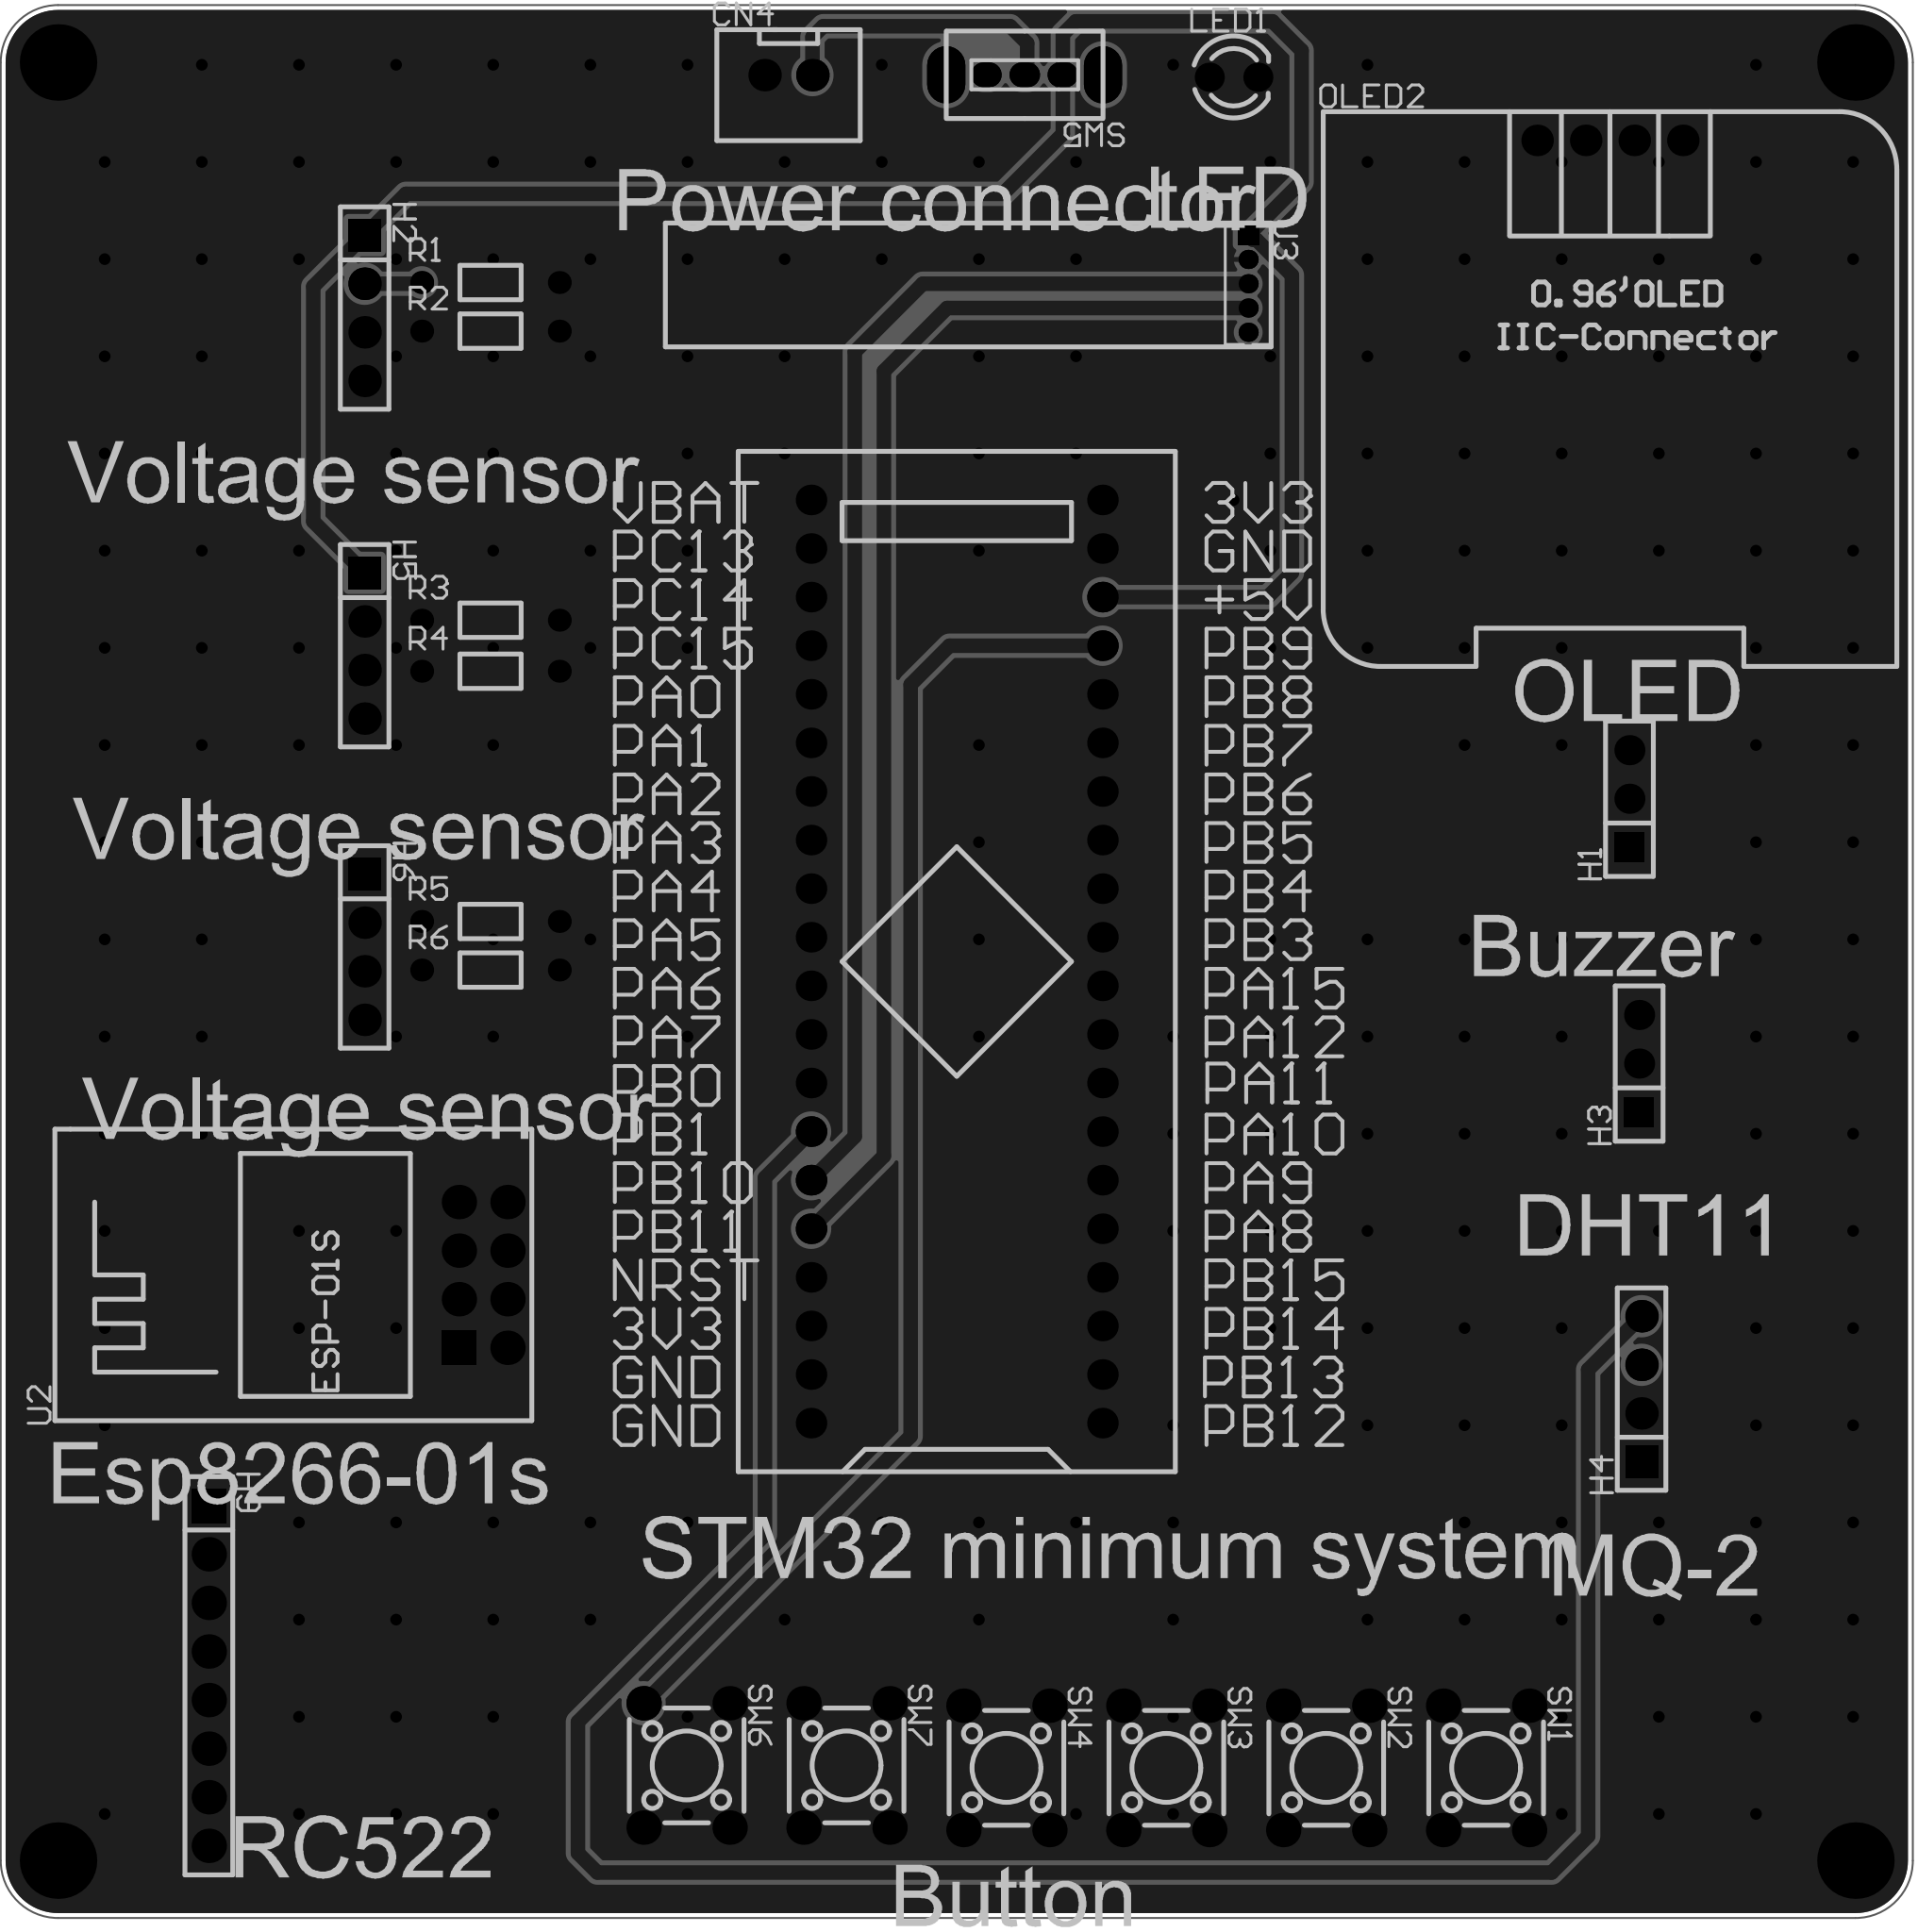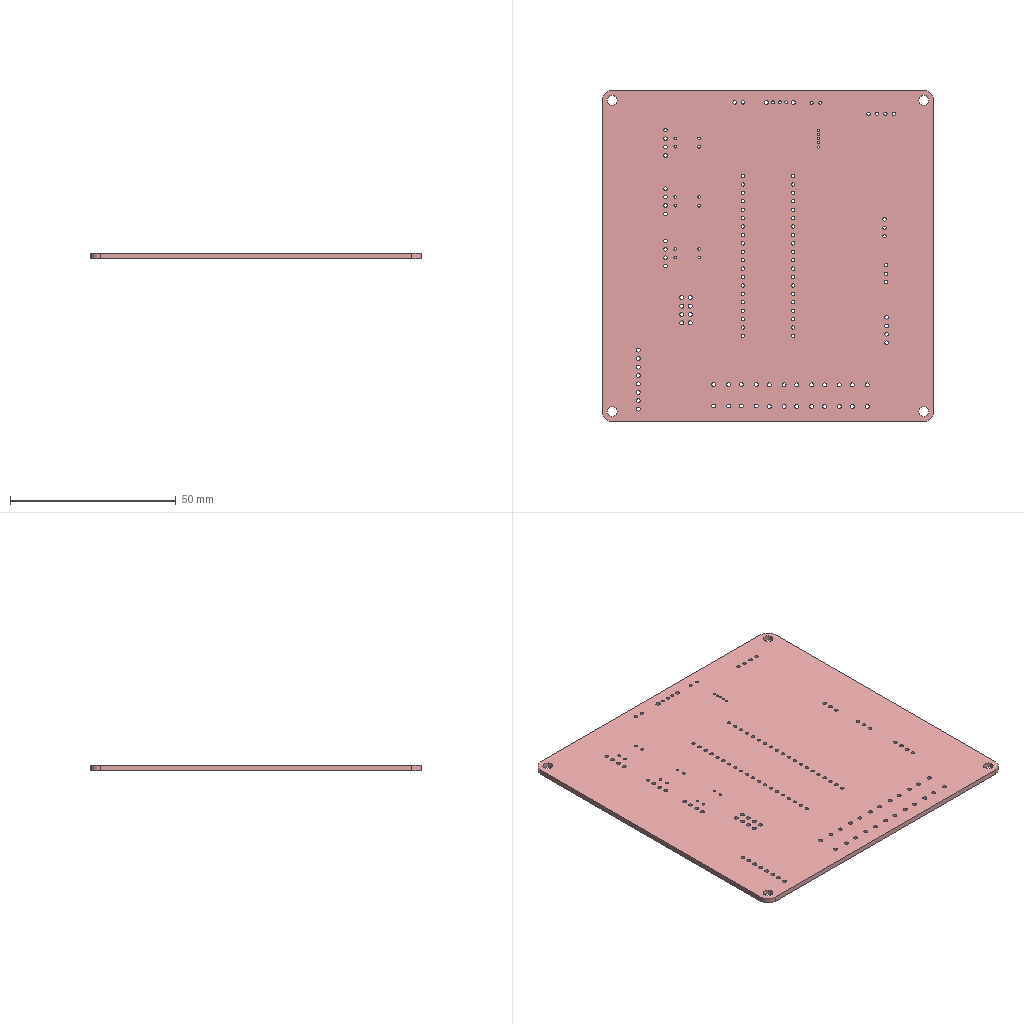Circuit board layout | Altium Designer | box 100 x 100 x 1.6 mm
Layer stack:
# Altium Designer layer stack of  (unit mm; dielectric type: 0 none, 1 core, 2 prepreg, 3 surface material)
index,name,kind,layer,copper_thickness_mm,dielectric_type,dielectric_thickness_mm,dielectric_material,dielectric_constant
0,Top Paste Mask Layer,other,,,,,,
1,Top Silkscreen Layer,other,,,,,,
2,Top Solder Mask Layer,dielectric,,,3,0.01,,3.3
3,Top Layer,copper,Top Layer,0.035,,,,
4,Dielectric1,dielectric,,,3,1.51,FR4,4.5
5,Bottom Layer,copper,Bottom Layer,0.035,,,,
6,Bottom Solder Mask Layer,dielectric,,,3,0.01,,3.3
7,Bottom Silkscreen Layer,other,,,,,,
8,Bottom Paste Mask Layer,other,,,,,,
# drill layer pairs: low layer,high layer
drill_pair,Top Layer,Bottom Layer
Part placement:
Designator,Comment,Layer,Footprint,Center-X(mm),Center-Y(mm),Rotation
U1,STM32F103C8T6-Card,TopLayer,CONN-TH_L53.3-W22.9_STM32F103C8T6-CARD,141.351,130.937,90
CN4,XH2.54*2P_THT,TopLayer,CONN-TH_2P-P2.50-XH2.54-2P,132.552,177.275,0
H1,,TopLayer,HDR-TH_3P-P2.54-V-F,176.53,139.446,90
H2,,TopLayer,HDR-TH_4P-P2.54-V-F,110.383,165.1,270
H3,,TopLayer,HDR-TH_3P-P2.54-V-F,177.038,125.603,90
H4,,TopLayer,HDR-TH_4P-P2.54-V-F,177.165,108.585,90
H5,,TopLayer,HDR-TH_4P-P2.54-V-F,110.383,147.447,270
H6,,TopLayer,HDR-TH_4P-P2.54-V-F,110.383,131.699,270
H9,,TopLayer,HDR-TH_8P-P2.54-V-F-1,102.235,93.599,270
LED1,,TopLayer,LED_TH-3mm,155.829,177.165,0
OLED2,,TopLayer,0.96OLED_4P,175.514,173.863,0
R1,10kΩ,TopLayer,Res_1/8W,116.967,166.433,0
R2,6.8kΩ,TopLayer,Res_1/8W,116.967,163.893,0
R3,10kΩ,TopLayer,Res_1/8W,116.967,148.78,0
R4,6.8kΩ,TopLayer,Res_1/8W,116.967,146.113,0
R5,10kΩ,TopLayer,Res_1/8W,116.967,133.032,0
R6,6.8kΩ,TopLayer,Res_1/8W,116.967,130.492,0
SW1,,TopLayer,SW-TH_4P-L6.0-W6.0-P4.50-LS6.5,169.036,88.785,270
SW2,,TopLayer,SW-TH_4P-L6.0-W6.0-P4.50-LS6.5,160.673,88.785,270
SW3,,TopLayer,SW-TH_4P-L6.0-W6.0-P4.50-LS6.5,152.311,88.785,270
SW4,,TopLayer,SW-TH_4P-L6.0-W6.0-P4.50-LS6.5,143.949,88.785,270
SW5,,TopLayer,拨动开关,144.899,177.292,180
SW6,,TopLayer,SW-TH_4P-L6.0-W6.0-P4.50-LS6.5,127.224,88.912,270
SW7,,TopLayer,SW-TH_4P-L6.0-W6.0-P4.50-LS6.5,135.587,88.912,270
U2,ESP-01S,TopLayer,WIFIM-TH_ESP-01S,116.586,114.554,90
U3,FPH12728-S05S1014190140B,TopLayer,HDR-TH_5P-P1.27-V-M-1,156.591,166.37,270
Pad and via stacks:
# Altium Designer via and pad stacks of  (unit mm). Each distinct definition once, with the count of objects using it.
# via: kind,start_layer,end_layer,hole_mm,diameter_mm,mode(0 simple;1 top-mid-bottom;2 full stack),diameter_per_layer,count,example_net
# pad: kind,layer,hole_mm,hole_type(0 round;1 square;2 slot),plating,top_size,top_shape(1 round;2 rect;3 octagon;9 rounded rect),mid_size,bottom_size,mode,footprint,size_per_layer,count,example
pad,Multi-Layer,3,0,plated,4x4,1,4x4,4x4,0,,,4,1
pad,Multi-Layer,1,0,plated,1.6x1.6,1,1.6x1.6,1.6x1.6,0,CONN-TH_L53.3-W22.9_STM32F103C8T6-CARD,,40,U1.1
pad,Multi-Layer,1.05,0,plated,1.7x1.7,1,1.7x1.7,1.7x1.7,0,CONN-TH_2P-P2.50-XH2.54-2P,,2,CN4.2
pad,Multi-Layer,1.02,0,plated,1.575x1.575,1,1.575x1.575,1.575x1.575,0,HDR-TH_3P-P2.54-V-F,,4,H1.3
pad,Multi-Layer,1.02,0,plated,1.575x1.575,2,1.575x1.575,1.575x1.575,0,HDR-TH_3P-P2.54-V-F,,2,H1.1
pad,Multi-Layer,1.1,0,plated,1.7x1.7,2,1.7x1.7,1.7x1.7,0,HDR-TH_4P-P2.54-V-F,,4,H2.1
pad,Multi-Layer,1.1,0,plated,1.7x1.7,1,1.7x1.7,1.7x1.7,0,HDR-TH_4P-P2.54-V-F,,12,H2.2
pad,Multi-Layer,1.2,0,plated,1.8x1.8,2,1.8x1.8,1.8x1.8,0,HDR-TH_8P-P2.54-V-F-1,,1,H9.1
pad,Multi-Layer,1.2,0,plated,1.8x1.8,1,1.8x1.8,1.8x1.8,0,HDR-TH_8P-P2.54-V-F-1,,7,H9.2
pad,Multi-Layer,0.9144,0,plated,1.524x1.524,1,1.524x1.524,1.524x1.524,0,LED_TH-3mm,,2,LED1.1
pad,Multi-Layer,1,0,plated,1.65x1.65,1,1.65x1.65,1.65x1.65,0,0.96OLED_4P,,4,OLED2.4
pad,Multi-Layer,0.8001,0,plated,1.199x1.199,1,1.199x1.199,1.199x1.199,0,Res_1/8W,,12,R1.1
pad,Multi-Layer,1.2,0,plated,1.8x1.8,1,1.8x1.8,1.8x1.8,0,SW-TH_4P-L6.0-W6.0-P4.50-LS6.5,,24,SW1.1
pad,Multi-Layer,0.8992,0,plated,1.6x1.3,1,1.6x1.3,1.6x1.3,0,\u00B2\u00A6\u00B6\u00AF\u00BF\u00AA\u00B9\u00D8,,3,SW5.1
pad,Multi-Layer,1.3,0,plated,3x1.999,1,3x1.999,3x1.999,0,\u00B2\u00A6\u00B6\u00AF\u00BF\u00AA\u00B9\u00D8,,2,SW5.4
pad,Multi-Layer,1.2,0,plated,1.8x1.8,2,1.8x1.8,1.8x1.8,0,WIFIM-TH_ESP-01S,,1,U2.1
pad,Multi-Layer,1.2,0,plated,1.8x1.8,1,1.8x1.8,1.8x1.8,0,WIFIM-TH_ESP-01S,,7,U2.2
pad,Multi-Layer,0.65,0,plated,1x1,1,1x1,1x1,0,HDR-TH_5P-P1.27-V-M-1,,4,U3.5
pad,Multi-Layer,0.65,0,plated,1x1.1,2,1x1.1,1x1.1,0,HDR-TH_5P-P1.27-V-M-1,,1,U3.1
via,Top Layer,Bottom Layer,0.3048,0.61,0,,226,VCC
Copper pours:
name,layer,net,type(0 solid;1 hatched;2 none)
Bottom Layer-GND,Bottom Layer,GND,0
Top Layer-GND,Top Layer,GND,0
Design rules, without the lines most boards share:
# Altium Designer design rules of  (exported by Altium Designer, unit mm)
# columns: name | kind | enabled | priority | scope1 | scope2 | descriptor | typed fields (field=value)
Copper_copperRegion_copperThickness1oz | 0 | disabled | 4 | All | All | Clearance Constraint (Gap=5.984mil) (Disabled)(All),(All) | gap=0.152
Copper_copperRegion_copperThickness1oz_1 | 63 | disabled | 4 | All | All | Board Clearance Constraint (Gap=0mil) (Disabled)(All) |
Copper_copperRegion_Copper_copperRegion | 0 | disabled | 5 | All | All | Clearance Constraint (Gap=5.984mil) (Disabled)(All),(All) | gap=0.152
Copper_copperRegion_Copper_copperRegion_1 | 63 | disabled | 5 | All | All | Board Clearance Constraint (Gap=0mil) (Disabled)(All) |
copperThickness1oz | 0 | enabled | 6 | All | All | Clearance Constraint (Gap=5.984mil) (All),(All) | gap=0.152
copperThickness1oz_1 | 63 | enabled | 6 | All | All | Board Clearance Constraint (Gap=0mil) (All) |
copperRegion_copperThickness1oz | 20 | disabled | 1 | All | All | Polygon Connect Rule(Relief Connect )(Conductor Width=10mil) (Relief Angle=90 Angle) (Entries=4) (Air Gap Width=10mil) (Disabled)(All),(All) | connect_style(0=relief,1=direct,2=none)=0 relief_conductor_width=0.254 relief_entries=4
copperRegion_Copper_copperRegion | 20 | disabled | 2 | All | All | Polygon Connect Rule(Relief Connect )(Conductor Width=10mil) (Relief Angle=90 Angle) (Entries=4) (Air Gap Width=10mil) (Disabled)(All),(All) | connect_style(0=relief,1=direct,2=none)=0 relief_conductor_width=0.254 relief_entries=4
copperRegion | 20 | enabled | 3 | All | All | Polygon Connect Rule(Relief Connect )(Conductor Width=10mil) (Relief Angle=90 Angle) (Entries=4) (Air Gap Width=10mil) (All),(All) | connect_style(0=relief,1=direct,2=none)=0 relief_conductor_width=0.254 relief_entries=4